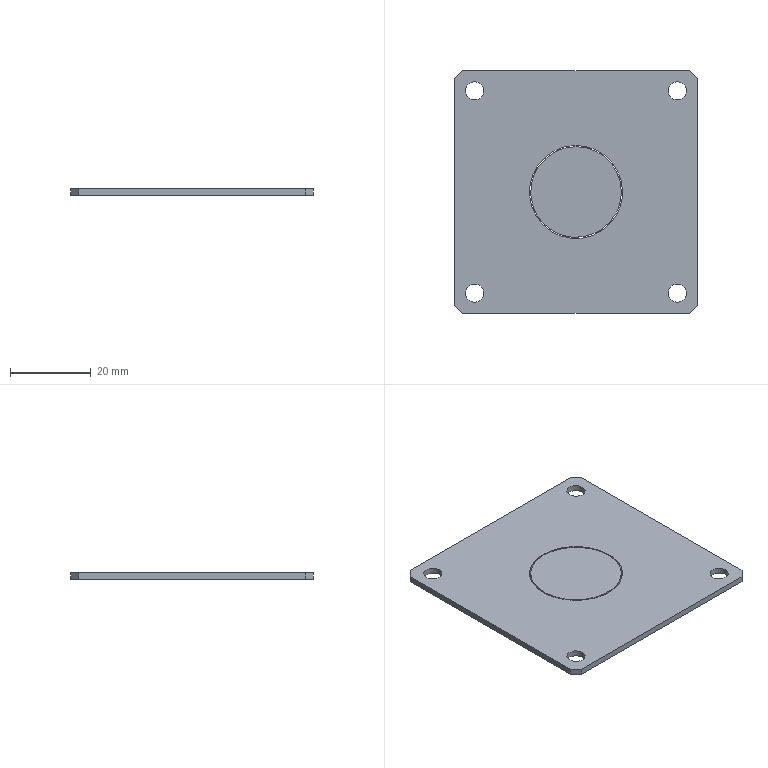Part | STEP file | 接头2 | 1 solid | 32 faces | box 60 x 60 x 1.5 mm | volume 5261 mm3 | cylinder 16 | plane 16 | commonest cylinder face diameters 4.5 x8 22.4 x4 23 x4